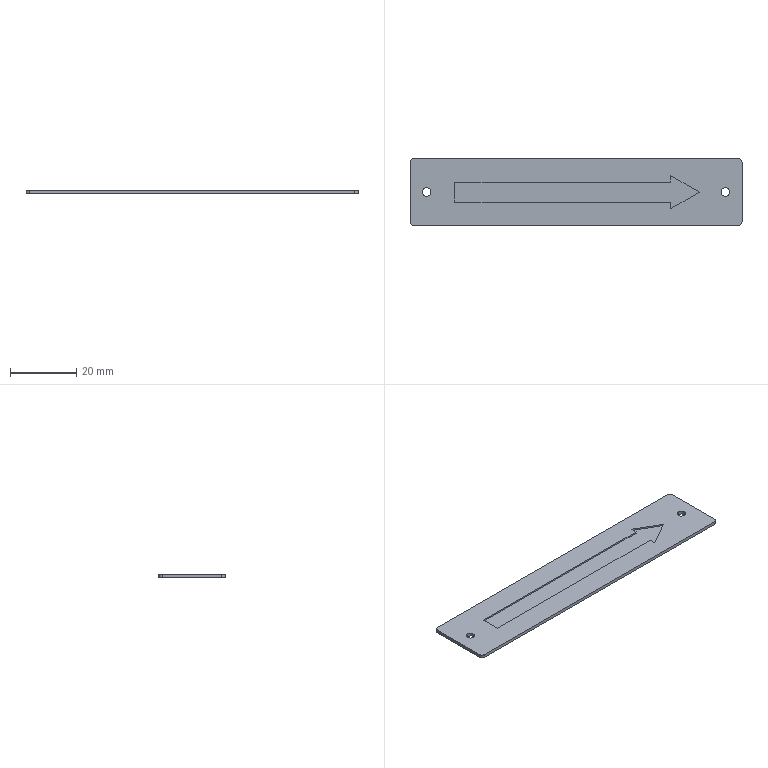Part | STEP file | [Flow direction nameplate]-Part-2 | 1 solid | 22 faces | box 100 x 20 x 1 mm | volume 1794 mm3 | plane 14 | cylinder 8 | commonest cylinder face diameters 2 x4 2.5 x4
STEP:
#1=CARTESIAN_POINT('',(-320.023,-38.283,51.8));
#2=VERTEX_POINT('',#1);
#3=CARTESIAN_POINT('',(-320.023,-35.783,51.8));
#4=VERTEX_POINT('',#3);
#5=CARTESIAN_POINT('',(-320.023,-37.033,51.8));
#6=DIRECTION('',(0.,0.,-1.));
#7=DIRECTION('',(0.,1.,0.));
#8=AXIS2_PLACEMENT_3D('',#5,#6,#7);
#9=CIRCLE('',#8,1.25);
#10=EDGE_CURVE('',#2,#4,#9,.T.);
#11=ORIENTED_EDGE('',*,*,#10,.F.);
#12=CARTESIAN_POINT('',(-320.023,-38.283,50.8));
#13=VERTEX_POINT('',#12);
#14=CARTESIAN_POINT('',(-320.023,-38.283,51.8));
#15=DIRECTION('',(0.,0.,-1.));
#16=VECTOR('',#15,1000.);
#17=LINE('',#14,#16);
#18=EDGE_CURVE('',#2,#13,#17,.T.);
#19=ORIENTED_EDGE('',*,*,#18,.T.);
#20=CARTESIAN_POINT('',(-320.023,-35.783,50.8));
#21=VERTEX_POINT('',#20);
#22=CARTESIAN_POINT('',(-320.023,-37.033,50.8));
#23=DIRECTION('',(0.,0.,1.));
#24=DIRECTION('',(0.,-1.,0.));
#25=AXIS2_PLACEMENT_3D('',#22,#23,#24);
#26=CIRCLE('',#25,1.25);
#27=EDGE_CURVE('',#21,#13,#26,.T.);
#28=ORIENTED_EDGE('',*,*,#27,.F.);
#29=CARTESIAN_POINT('',(-320.023,-35.783,51.8));
#30=DIRECTION('',(0.,0.,-1.));
#31=VECTOR('',#30,1000.);
#32=LINE('',#29,#31);
#33=EDGE_CURVE('',#4,#21,#32,.T.);
#34=ORIENTED_EDGE('',*,*,#33,.F.);
#35=EDGE_LOOP('',(#11,#19,#28,#34));
#36=FACE_OUTER_BOUND('',#35,.T.);
#37=CARTESIAN_POINT('',(-320.023,-37.033,51.8));
#38=DIRECTION('',(0.,0.,-1.));
#39=DIRECTION('',(0.,1.,0.));
#40=AXIS2_PLACEMENT_3D('',#37,#38,#39);
#41=CYLINDRICAL_SURFACE('',#40,1.25);
#42=ADVANCED_FACE('',(#36),#41,.F.);
#43=CARTESIAN_POINT('',(-230.023,-38.283,51.8));
#44=VERTEX_POINT('',#43);
#45=CARTESIAN_POINT('',(-230.023,-35.783,51.8));
#46=VERTEX_POINT('',#45);
#47=CARTESIAN_POINT('',(-230.023,-37.033,51.8));
#48=DIRECTION('',(0.,0.,-1.));
#49=DIRECTION('',(0.,1.,0.));
#50=AXIS2_PLACEMENT_3D('',#47,#48,#49);
#51=CIRCLE('',#50,1.25);
#52=EDGE_CURVE('',#44,#46,#51,.T.);
#53=ORIENTED_EDGE('',*,*,#52,.F.);
#54=CARTESIAN_POINT('',(-230.023,-38.283,50.8));
#55=VERTEX_POINT('',#54);
#56=CARTESIAN_POINT('',(-230.023,-38.283,51.8));
#57=DIRECTION('',(0.,0.,-1.));
#58=VECTOR('',#57,1000.);
#59=LINE('',#56,#58);
#60=EDGE_CURVE('',#44,#55,#59,.T.);
#61=ORIENTED_EDGE('',*,*,#60,.T.);
#62=CARTESIAN_POINT('',(-230.023,-35.783,50.8));
#63=VERTEX_POINT('',#62);
#64=CARTESIAN_POINT('',(-230.023,-37.033,50.8));
#65=DIRECTION('',(0.,0.,1.));
#66=DIRECTION('',(0.,-1.,0.));
#67=AXIS2_PLACEMENT_3D('',#64,#65,#66);
#68=CIRCLE('',#67,1.25);
#69=EDGE_CURVE('',#63,#55,#68,.T.);
#70=ORIENTED_EDGE('',*,*,#69,.F.);
#71=CARTESIAN_POINT('',(-230.023,-35.783,51.8));
#72=DIRECTION('',(0.,0.,-1.));
#73=VECTOR('',#72,1000.);
#74=LINE('',#71,#73);
#75=EDGE_CURVE('',#46,#63,#74,.T.);
#76=ORIENTED_EDGE('',*,*,#75,.F.);
#77=EDGE_LOOP('',(#53,#61,#70,#76));
#78=FACE_OUTER_BOUND('',#77,.T.);
#79=CARTESIAN_POINT('',(-230.023,-37.033,51.8));
#80=DIRECTION('',(0.,0.,-1.));
#81=DIRECTION('',(0.,1.,0.));
#82=AXIS2_PLACEMENT_3D('',#79,#80,#81);
#83=CYLINDRICAL_SURFACE('',#82,1.25);
#84=ADVANCED_FACE('',(#78),#83,.F.);
#85=CARTESIAN_POINT('',(-324.023,-27.033,50.8));
#86=VERTEX_POINT('',#85);
#87=CARTESIAN_POINT('',(-226.023,-27.033,50.8));
#88=VERTEX_POINT('',#87);
#89=CARTESIAN_POINT('',(-275.023,-27.033,50.8));
#90=DIRECTION('',(1.,0.,0.));
#91=VECTOR('',#90,1000.);
#92=LINE('',#89,#91);
#93=EDGE_CURVE('',#86,#88,#92,.T.);
#94=ORIENTED_EDGE('',*,*,#93,.F.);
#95=CARTESIAN_POINT('',(-324.023,-27.033,51.8));
#96=VERTEX_POINT('',#95);
#97=CARTESIAN_POINT('',(-324.023,-27.033,51.3));
#98=DIRECTION('',(0.,0.,1.));
#99=VECTOR('',#98,1000.);
#100=LINE('',#97,#99);
#101=EDGE_CURVE('',#86,#96,#100,.T.);
#102=ORIENTED_EDGE('',*,*,#101,.T.);
#103=CARTESIAN_POINT('',(-226.023,-27.033,51.8));
#104=VERTEX_POINT('',#103);
#105=CARTESIAN_POINT('',(-275.023,-27.033,51.8));
#106=DIRECTION('',(-1.,0.,0.));
#107=VECTOR('',#106,1000.);
#108=LINE('',#105,#107);
#109=EDGE_CURVE('',#104,#96,#108,.T.);
#110=ORIENTED_EDGE('',*,*,#109,.F.);
#111=CARTESIAN_POINT('',(-226.023,-27.033,51.3));
#112=DIRECTION('',(0.,0.,-1.));
#113=VECTOR('',#112,1000.);
#114=LINE('',#111,#113);
#115=EDGE_CURVE('',#104,#88,#114,.T.);
#116=ORIENTED_EDGE('',*,*,#115,.T.);
#117=EDGE_LOOP('',(#94,#102,#110,#116));
#118=FACE_OUTER_BOUND('',#117,.T.);
#119=CARTESIAN_POINT('',(-275.023,-27.033,51.3));
#120=DIRECTION('',(0.,1.,0.));
#121=DIRECTION('',(1.,0.,0.));
#122=AXIS2_PLACEMENT_3D('',#119,#120,#121);
#123=PLANE('',#122);
#124=ADVANCED_FACE('',(#118),#123,.T.);
#125=CARTESIAN_POINT('',(-311.498,-40.081,51.8));
#126=VERTEX_POINT('',#125);
#127=CARTESIAN_POINT('',(-311.498,-34.081,51.8));
#128=VERTEX_POINT('',#127);
#129=CARTESIAN_POINT('',(-311.498,-47.033,51.8));
#130=DIRECTION('',(0.,1.,0.));
#131=VECTOR('',#130,1000.);
#132=LINE('',#129,#131);
#133=EDGE_CURVE('',#126,#128,#132,.T.);
#134=ORIENTED_EDGE('',*,*,#133,.T.);
#135=CARTESIAN_POINT('',(-246.498,-34.081,51.8));
#136=VERTEX_POINT('',#135);
#137=CARTESIAN_POINT('',(-275.023,-34.081,51.8));
#138=DIRECTION('',(1.,0.,0.));
#139=VECTOR('',#138,1000.);
#140=LINE('',#137,#139);
#141=EDGE_CURVE('',#128,#136,#140,.T.);
#142=ORIENTED_EDGE('',*,*,#141,.T.);
#143=CARTESIAN_POINT('',(-246.498,-32.081,51.8));
#144=VERTEX_POINT('',#143);
#145=CARTESIAN_POINT('',(-246.498,-47.033,51.8));
#146=DIRECTION('',(0.,1.,0.));
#147=VECTOR('',#146,1000.);
#148=LINE('',#145,#147);
#149=EDGE_CURVE('',#136,#144,#148,.T.);
#150=ORIENTED_EDGE('',*,*,#149,.T.);
#151=CARTESIAN_POINT('',(-237.838,-37.081,51.8));
#152=VERTEX_POINT('',#151);
#153=CARTESIAN_POINT('',(-261.417,-23.467,51.8));
#154=DIRECTION('',(0.866,-0.5,0.));
#155=VECTOR('',#154,1000.);
#156=LINE('',#153,#155);
#157=EDGE_CURVE('',#144,#152,#156,.T.);
#158=ORIENTED_EDGE('',*,*,#157,.T.);
#159=CARTESIAN_POINT('',(-246.498,-42.081,51.8));
#160=VERTEX_POINT('',#159);
#161=CARTESIAN_POINT('',(-270.036,-55.67,51.8));
#162=DIRECTION('',(-0.866,-0.5,0.));
#163=VECTOR('',#162,1000.);
#164=LINE('',#161,#163);
#165=EDGE_CURVE('',#152,#160,#164,.T.);
#166=ORIENTED_EDGE('',*,*,#165,.T.);
#167=CARTESIAN_POINT('',(-246.498,-40.081,51.8));
#168=VERTEX_POINT('',#167);
#169=CARTESIAN_POINT('',(-246.498,-47.033,51.8));
#170=DIRECTION('',(0.,1.,0.));
#171=VECTOR('',#170,1000.);
#172=LINE('',#169,#171);
#173=EDGE_CURVE('',#160,#168,#172,.T.);
#174=ORIENTED_EDGE('',*,*,#173,.T.);
#175=CARTESIAN_POINT('',(-275.023,-40.081,51.8));
#176=DIRECTION('',(-1.,0.,0.));
#177=VECTOR('',#176,1000.);
#178=LINE('',#175,#177);
#179=EDGE_CURVE('',#168,#126,#178,.T.);
#180=ORIENTED_EDGE('',*,*,#179,.T.);
#181=EDGE_LOOP('',(#134,#142,#150,#158,#166,#174,#180));
#182=FACE_BOUND('',#181,.T.);
#183=CARTESIAN_POINT('',(-320.023,-37.033,51.8));
#184=DIRECTION('',(0.,0.,-1.));
#185=DIRECTION('',(0.,1.,0.));
#186=AXIS2_PLACEMENT_3D('',#183,#184,#185);
#187=CIRCLE('',#186,1.25);
#188=EDGE_CURVE('',#4,#2,#187,.T.);
#189=ORIENTED_EDGE('',*,*,#188,.T.);
#190=ORIENTED_EDGE('',*,*,#10,.T.);
#191=EDGE_LOOP('',(#189,#190));
#192=FACE_BOUND('',#191,.T.);
#193=CARTESIAN_POINT('',(-230.023,-37.033,51.8));
#194=DIRECTION('',(0.,0.,-1.));
#195=DIRECTION('',(0.,1.,0.));
#196=AXIS2_PLACEMENT_3D('',#193,#194,#195);
#197=CIRCLE('',#196,1.25);
#198=EDGE_CURVE('',#46,#44,#197,.T.);
#199=ORIENTED_EDGE('',*,*,#198,.T.);
#200=ORIENTED_EDGE('',*,*,#52,.T.);
#201=EDGE_LOOP('',(#199,#200));
#202=FACE_BOUND('',#201,.T.);
#203=CARTESIAN_POINT('',(-325.023,-46.033,51.8));
#204=VERTEX_POINT('',#203);
#205=CARTESIAN_POINT('',(-325.023,-28.033,51.8));
#206=VERTEX_POINT('',#205);
#207=CARTESIAN_POINT('',(-325.023,-47.033,51.8));
#208=DIRECTION('',(0.,1.,0.));
#209=VECTOR('',#208,1000.);
#210=LINE('',#207,#209);
#211=EDGE_CURVE('',#204,#206,#210,.T.);
#212=ORIENTED_EDGE('',*,*,#211,.F.);
#213=CARTESIAN_POINT('',(-324.023,-47.033,51.8));
#214=VERTEX_POINT('',#213);
#215=CARTESIAN_POINT('',(-324.023,-46.033,51.8));
#216=DIRECTION('',(0.,0.,1.));
#217=DIRECTION('',(0.,-1.,0.));
#218=AXIS2_PLACEMENT_3D('',#215,#216,#217);
#219=CIRCLE('',#218,1.);
#220=EDGE_CURVE('',#204,#214,#219,.T.);
#221=ORIENTED_EDGE('',*,*,#220,.T.);
#222=CARTESIAN_POINT('',(-226.023,-47.033,51.8));
#223=VERTEX_POINT('',#222);
#224=CARTESIAN_POINT('',(-275.023,-47.033,51.8));
#225=DIRECTION('',(1.,0.,0.));
#226=VECTOR('',#225,1000.);
#227=LINE('',#224,#226);
#228=EDGE_CURVE('',#214,#223,#227,.T.);
#229=ORIENTED_EDGE('',*,*,#228,.T.);
#230=CARTESIAN_POINT('',(-225.023,-46.033,51.8));
#231=VERTEX_POINT('',#230);
#232=CARTESIAN_POINT('',(-226.023,-46.033,51.8));
#233=DIRECTION('',(0.,0.,1.));
#234=DIRECTION('',(0.,-1.,0.));
#235=AXIS2_PLACEMENT_3D('',#232,#233,#234);
#236=CIRCLE('',#235,1.);
#237=EDGE_CURVE('',#223,#231,#236,.T.);
#238=ORIENTED_EDGE('',*,*,#237,.T.);
#239=CARTESIAN_POINT('',(-225.023,-28.033,51.8));
#240=VERTEX_POINT('',#239);
#241=CARTESIAN_POINT('',(-225.023,-47.033,51.8));
#242=DIRECTION('',(0.,1.,0.));
#243=VECTOR('',#242,1000.);
#244=LINE('',#241,#243);
#245=EDGE_CURVE('',#231,#240,#244,.T.);
#246=ORIENTED_EDGE('',*,*,#245,.T.);
#247=CARTESIAN_POINT('',(-226.023,-28.033,51.8));
#248=DIRECTION('',(0.,0.,1.));
#249=DIRECTION('',(0.,-1.,0.));
#250=AXIS2_PLACEMENT_3D('',#247,#248,#249);
#251=CIRCLE('',#250,1.);
#252=EDGE_CURVE('',#240,#104,#251,.T.);
#253=ORIENTED_EDGE('',*,*,#252,.T.);
#254=ORIENTED_EDGE('',*,*,#109,.T.);
#255=CARTESIAN_POINT('',(-324.023,-28.033,51.8));
#256=DIRECTION('',(0.,0.,1.));
#257=DIRECTION('',(0.,-1.,0.));
#258=AXIS2_PLACEMENT_3D('',#255,#256,#257);
#259=CIRCLE('',#258,1.);
#260=EDGE_CURVE('',#96,#206,#259,.T.);
#261=ORIENTED_EDGE('',*,*,#260,.T.);
#262=EDGE_LOOP('',(#212,#221,#229,#238,#246,#253,#254,#261));
#263=FACE_OUTER_BOUND('',#262,.T.);
#264=CARTESIAN_POINT('',(-275.023,-47.033,51.8));
#265=DIRECTION('',(0.,0.,1.));
#266=DIRECTION('',(0.,-1.,0.));
#267=AXIS2_PLACEMENT_3D('',#264,#265,#266);
#268=PLANE('',#267);
#269=ADVANCED_FACE('',(#182,#192,#202,#263),#268,.T.);
#270=CARTESIAN_POINT('',(-325.023,-46.033,50.8));
#271=VERTEX_POINT('',#270);
#272=CARTESIAN_POINT('',(-325.023,-28.033,50.8));
#273=VERTEX_POINT('',#272);
#274=CARTESIAN_POINT('',(-325.023,-47.033,50.8));
#275=DIRECTION('',(0.,1.,0.));
#276=VECTOR('',#275,1000.);
#277=LINE('',#274,#276);
#278=EDGE_CURVE('',#271,#273,#277,.T.);
#279=ORIENTED_EDGE('',*,*,#278,.F.);
#280=CARTESIAN_POINT('',(-325.023,-46.033,51.3));
#281=DIRECTION('',(0.,0.,1.));
#282=VECTOR('',#281,1000.);
#283=LINE('',#280,#282);
#284=EDGE_CURVE('',#271,#204,#283,.T.);
#285=ORIENTED_EDGE('',*,*,#284,.T.);
#286=ORIENTED_EDGE('',*,*,#211,.T.);
#287=CARTESIAN_POINT('',(-325.023,-28.033,51.3));
#288=DIRECTION('',(0.,0.,-1.));
#289=VECTOR('',#288,1000.);
#290=LINE('',#287,#289);
#291=EDGE_CURVE('',#206,#273,#290,.T.);
#292=ORIENTED_EDGE('',*,*,#291,.T.);
#293=EDGE_LOOP('',(#279,#285,#286,#292));
#294=FACE_OUTER_BOUND('',#293,.T.);
#295=CARTESIAN_POINT('',(-325.023,-47.033,51.3));
#296=DIRECTION('',(-1.,0.,0.));
#297=DIRECTION('',(0.,1.,0.));
#298=AXIS2_PLACEMENT_3D('',#295,#296,#297);
#299=PLANE('',#298);
#300=ADVANCED_FACE('',(#294),#299,.T.);
#301=ORIENTED_EDGE('',*,*,#27,.T.);
#302=CARTESIAN_POINT('',(-320.023,-37.033,50.8));
#303=DIRECTION('',(0.,0.,1.));
#304=DIRECTION('',(0.,-1.,0.));
#305=AXIS2_PLACEMENT_3D('',#302,#303,#304);
#306=CIRCLE('',#305,1.25);
#307=EDGE_CURVE('',#13,#21,#306,.T.);
#308=ORIENTED_EDGE('',*,*,#307,.T.);
#309=EDGE_LOOP('',(#301,#308));
#310=FACE_BOUND('',#309,.T.);
#311=ORIENTED_EDGE('',*,*,#69,.T.);
#312=CARTESIAN_POINT('',(-230.023,-37.033,50.8));
#313=DIRECTION('',(0.,0.,1.));
#314=DIRECTION('',(0.,-1.,0.));
#315=AXIS2_PLACEMENT_3D('',#312,#313,#314);
#316=CIRCLE('',#315,1.25);
#317=EDGE_CURVE('',#55,#63,#316,.T.);
#318=ORIENTED_EDGE('',*,*,#317,.T.);
#319=EDGE_LOOP('',(#311,#318));
#320=FACE_BOUND('',#319,.T.);
#321=CARTESIAN_POINT('',(-226.023,-47.033,50.8));
#322=VERTEX_POINT('',#321);
#323=CARTESIAN_POINT('',(-324.023,-47.033,50.8));
#324=VERTEX_POINT('',#323);
#325=CARTESIAN_POINT('',(-275.023,-47.033,50.8));
#326=DIRECTION('',(-1.,0.,0.));
#327=VECTOR('',#326,1000.);
#328=LINE('',#325,#327);
#329=EDGE_CURVE('',#322,#324,#328,.T.);
#330=ORIENTED_EDGE('',*,*,#329,.T.);
#331=CARTESIAN_POINT('',(-324.023,-46.033,50.8));
#332=DIRECTION('',(0.,0.,-1.));
#333=DIRECTION('',(0.,1.,0.));
#334=AXIS2_PLACEMENT_3D('',#331,#332,#333);
#335=CIRCLE('',#334,1.);
#336=EDGE_CURVE('',#324,#271,#335,.T.);
#337=ORIENTED_EDGE('',*,*,#336,.T.);
#338=ORIENTED_EDGE('',*,*,#278,.T.);
#339=CARTESIAN_POINT('',(-324.023,-28.033,50.8));
#340=DIRECTION('',(0.,0.,-1.));
#341=DIRECTION('',(0.,1.,0.));
#342=AXIS2_PLACEMENT_3D('',#339,#340,#341);
#343=CIRCLE('',#342,1.);
#344=EDGE_CURVE('',#273,#86,#343,.T.);
#345=ORIENTED_EDGE('',*,*,#344,.T.);
#346=ORIENTED_EDGE('',*,*,#93,.T.);
#347=CARTESIAN_POINT('',(-225.023,-28.033,50.8));
#348=VERTEX_POINT('',#347);
#349=CARTESIAN_POINT('',(-226.023,-28.033,50.8));
#350=DIRECTION('',(0.,0.,-1.));
#351=DIRECTION('',(0.,1.,0.));
#352=AXIS2_PLACEMENT_3D('',#349,#350,#351);
#353=CIRCLE('',#352,1.);
#354=EDGE_CURVE('',#88,#348,#353,.T.);
#355=ORIENTED_EDGE('',*,*,#354,.T.);
#356=CARTESIAN_POINT('',(-225.023,-46.033,50.8));
#357=VERTEX_POINT('',#356);
#358=CARTESIAN_POINT('',(-225.023,-47.033,50.8));
#359=DIRECTION('',(0.,1.,0.));
#360=VECTOR('',#359,1000.);
#361=LINE('',#358,#360);
#362=EDGE_CURVE('',#357,#348,#361,.T.);
#363=ORIENTED_EDGE('',*,*,#362,.F.);
#364=CARTESIAN_POINT('',(-226.023,-46.033,50.8));
#365=DIRECTION('',(0.,0.,-1.));
#366=DIRECTION('',(0.,1.,0.));
#367=AXIS2_PLACEMENT_3D('',#364,#365,#366);
#368=CIRCLE('',#367,1.);
#369=EDGE_CURVE('',#357,#322,#368,.T.);
#370=ORIENTED_EDGE('',*,*,#369,.T.);
#371=EDGE_LOOP('',(#330,#337,#338,#345,#346,#355,#363,#370));
#372=FACE_OUTER_BOUND('',#371,.T.);
#373=CARTESIAN_POINT('',(-275.023,-47.033,50.8));
#374=DIRECTION('',(0.,0.,-1.));
#375=DIRECTION('',(0.,1.,0.));
#376=AXIS2_PLACEMENT_3D('',#373,#374,#375);
#377=PLANE('',#376);
#378=ADVANCED_FACE('',(#310,#320,#372),#377,.T.);
#379=ORIENTED_EDGE('',*,*,#228,.F.);
#380=CARTESIAN_POINT('',(-324.023,-47.033,51.3));
#381=DIRECTION('',(0.,0.,-1.));
#382=VECTOR('',#381,1000.);
#383=LINE('',#380,#382);
#384=EDGE_CURVE('',#214,#324,#383,.T.);
#385=ORIENTED_EDGE('',*,*,#384,.T.);
#386=ORIENTED_EDGE('',*,*,#329,.F.);
#387=CARTESIAN_POINT('',(-226.023,-47.033,51.3));
#388=DIRECTION('',(0.,0.,1.));
#389=VECTOR('',#388,1000.);
#390=LINE('',#387,#389);
#391=EDGE_CURVE('',#322,#223,#390,.T.);
#392=ORIENTED_EDGE('',*,*,#391,.T.);
#393=EDGE_LOOP('',(#379,#385,#386,#392));
#394=FACE_OUTER_BOUND('',#393,.T.);
#395=CARTESIAN_POINT('',(-275.023,-47.033,51.3));
#396=DIRECTION('',(0.,-1.,0.));
#397=DIRECTION('',(-1.,0.,0.));
#398=AXIS2_PLACEMENT_3D('',#395,#396,#397);
#399=PLANE('',#398);
#400=ADVANCED_FACE('',(#394),#399,.T.);
#401=ORIENTED_EDGE('',*,*,#362,.T.);
#402=CARTESIAN_POINT('',(-225.023,-28.033,51.3));
#403=DIRECTION('',(0.,0.,1.));
#404=VECTOR('',#403,1000.);
#405=LINE('',#402,#404);
#406=EDGE_CURVE('',#348,#240,#405,.T.);
#407=ORIENTED_EDGE('',*,*,#406,.T.);
#408=ORIENTED_EDGE('',*,*,#245,.F.);
#409=CARTESIAN_POINT('',(-225.023,-46.033,51.3));
#410=DIRECTION('',(0.,0.,-1.));
#411=VECTOR('',#410,1000.);
#412=LINE('',#409,#411);
#413=EDGE_CURVE('',#231,#357,#412,.T.);
#414=ORIENTED_EDGE('',*,*,#413,.T.);
#415=EDGE_LOOP('',(#401,#407,#408,#414));
#416=FACE_OUTER_BOUND('',#415,.T.);
#417=CARTESIAN_POINT('',(-225.023,-47.033,51.3));
#418=DIRECTION('',(1.,0.,0.));
#419=DIRECTION('',(0.,-1.,0.));
#420=AXIS2_PLACEMENT_3D('',#417,#418,#419);
#421=PLANE('',#420);
#422=ADVANCED_FACE('',(#416),#421,.T.);
#423=ORIENTED_EDGE('',*,*,#60,.F.);
#424=ORIENTED_EDGE('',*,*,#198,.F.);
#425=ORIENTED_EDGE('',*,*,#75,.T.);
#426=ORIENTED_EDGE('',*,*,#317,.F.);
#427=EDGE_LOOP('',(#423,#424,#425,#426));
#428=FACE_OUTER_BOUND('',#427,.T.);
#429=CARTESIAN_POINT('',(-230.023,-37.033,51.8));
#430=DIRECTION('',(0.,0.,-1.));
#431=DIRECTION('',(0.,1.,0.));
#432=AXIS2_PLACEMENT_3D('',#429,#430,#431);
#433=CYLINDRICAL_SURFACE('',#432,1.25);
#434=ADVANCED_FACE('',(#428),#433,.F.);
#435=ORIENTED_EDGE('',*,*,#18,.F.);
#436=ORIENTED_EDGE('',*,*,#188,.F.);
#437=ORIENTED_EDGE('',*,*,#33,.T.);
#438=ORIENTED_EDGE('',*,*,#307,.F.);
#439=EDGE_LOOP('',(#435,#436,#437,#438));
#440=FACE_OUTER_BOUND('',#439,.T.);
#441=CARTESIAN_POINT('',(-320.023,-37.033,51.8));
#442=DIRECTION('',(0.,0.,-1.));
#443=DIRECTION('',(0.,1.,0.));
#444=AXIS2_PLACEMENT_3D('',#441,#442,#443);
#445=CYLINDRICAL_SURFACE('',#444,1.25);
#446=ADVANCED_FACE('',(#440),#445,.F.);
#447=ORIENTED_EDGE('',*,*,#237,.F.);
#448=ORIENTED_EDGE('',*,*,#391,.F.);
#449=ORIENTED_EDGE('',*,*,#369,.F.);
#450=ORIENTED_EDGE('',*,*,#413,.F.);
#451=EDGE_LOOP('',(#447,#448,#449,#450));
#452=FACE_OUTER_BOUND('',#451,.T.);
#453=CARTESIAN_POINT('',(-226.023,-46.033,51.3));
#454=DIRECTION('',(0.,0.,-1.));
#455=DIRECTION('',(0.,1.,0.));
#456=AXIS2_PLACEMENT_3D('',#453,#454,#455);
#457=CYLINDRICAL_SURFACE('',#456,1.);
#458=ADVANCED_FACE('',(#452),#457,.T.);
#459=ORIENTED_EDGE('',*,*,#354,.F.);
#460=ORIENTED_EDGE('',*,*,#115,.F.);
#461=ORIENTED_EDGE('',*,*,#252,.F.);
#462=ORIENTED_EDGE('',*,*,#406,.F.);
#463=EDGE_LOOP('',(#459,#460,#461,#462));
#464=FACE_OUTER_BOUND('',#463,.T.);
#465=CARTESIAN_POINT('',(-226.023,-28.033,51.3));
#466=DIRECTION('',(0.,0.,1.));
#467=DIRECTION('',(0.,-1.,0.));
#468=AXIS2_PLACEMENT_3D('',#465,#466,#467);
#469=CYLINDRICAL_SURFACE('',#468,1.);
#470=ADVANCED_FACE('',(#464),#469,.T.);
#471=ORIENTED_EDGE('',*,*,#260,.F.);
#472=ORIENTED_EDGE('',*,*,#101,.F.);
#473=ORIENTED_EDGE('',*,*,#344,.F.);
#474=ORIENTED_EDGE('',*,*,#291,.F.);
#475=EDGE_LOOP('',(#471,#472,#473,#474));
#476=FACE_OUTER_BOUND('',#475,.T.);
#477=CARTESIAN_POINT('',(-324.023,-28.033,51.3));
#478=DIRECTION('',(0.,0.,-1.));
#479=DIRECTION('',(0.,1.,0.));
#480=AXIS2_PLACEMENT_3D('',#477,#478,#479);
#481=CYLINDRICAL_SURFACE('',#480,1.);
#482=ADVANCED_FACE('',(#476),#481,.T.);
#483=ORIENTED_EDGE('',*,*,#336,.F.);
#484=ORIENTED_EDGE('',*,*,#384,.F.);
#485=ORIENTED_EDGE('',*,*,#220,.F.);
#486=ORIENTED_EDGE('',*,*,#284,.F.);
#487=EDGE_LOOP('',(#483,#484,#485,#486));
#488=FACE_OUTER_BOUND('',#487,.T.);
#489=CARTESIAN_POINT('',(-324.023,-46.033,51.3));
#490=DIRECTION('',(0.,0.,1.));
#491=DIRECTION('',(0.,-1.,0.));
#492=AXIS2_PLACEMENT_3D('',#489,#490,#491);
#493=CYLINDRICAL_SURFACE('',#492,1.);
#494=ADVANCED_FACE('',(#488),#493,.T.);
#495=ORIENTED_EDGE('',*,*,#133,.F.);
#496=CARTESIAN_POINT('',(-311.498,-40.081,51.35));
#497=VERTEX_POINT('',#496);
#498=CARTESIAN_POINT('',(-311.498,-40.081,51.85));
#499=DIRECTION('',(0.,0.,-1.));
#500=VECTOR('',#499,1000.);
#501=LINE('',#498,#500);
#502=EDGE_CURVE('',#126,#497,#501,.T.);
#503=ORIENTED_EDGE('',*,*,#502,.T.);
#504=CARTESIAN_POINT('',(-311.498,-34.081,51.35));
#505=VERTEX_POINT('',#504);
#506=CARTESIAN_POINT('',(-311.498,-34.081,51.35));
#507=DIRECTION('',(0.,-1.,0.));
#508=VECTOR('',#507,1000.);
#509=LINE('',#506,#508);
#510=EDGE_CURVE('',#505,#497,#509,.T.);
#511=ORIENTED_EDGE('',*,*,#510,.F.);
#512=CARTESIAN_POINT('',(-311.498,-34.081,51.85));
#513=DIRECTION('',(0.,0.,-1.));
#514=VECTOR('',#513,1000.);
#515=LINE('',#512,#514);
#516=EDGE_CURVE('',#128,#505,#515,.T.);
#517=ORIENTED_EDGE('',*,*,#516,.F.);
#518=EDGE_LOOP('',(#495,#503,#511,#517));
#519=FACE_OUTER_BOUND('',#518,.T.);
#520=CARTESIAN_POINT('',(-311.498,-34.081,51.85));
#521=DIRECTION('',(-1.,0.,0.));
#522=DIRECTION('',(0.,0.,-1.));
#523=AXIS2_PLACEMENT_3D('',#520,#521,#522);
#524=PLANE('',#523);
#525=ADVANCED_FACE('',(#519),#524,.F.);
#526=ORIENTED_EDGE('',*,*,#179,.F.);
#527=CARTESIAN_POINT('',(-246.498,-40.081,51.35));
#528=VERTEX_POINT('',#527);
#529=CARTESIAN_POINT('',(-246.498,-40.081,51.85));
#530=DIRECTION('',(0.,0.,-1.));
#531=VECTOR('',#530,1000.);
#532=LINE('',#529,#531);
#533=EDGE_CURVE('',#168,#528,#532,.T.);
#534=ORIENTED_EDGE('',*,*,#533,.T.);
#535=CARTESIAN_POINT('',(-311.498,-40.081,51.35));
#536=DIRECTION('',(1.,0.,0.));
#537=VECTOR('',#536,1000.);
#538=LINE('',#535,#537);
#539=EDGE_CURVE('',#497,#528,#538,.T.);
#540=ORIENTED_EDGE('',*,*,#539,.F.);
#541=ORIENTED_EDGE('',*,*,#502,.F.);
#542=EDGE_LOOP('',(#526,#534,#540,#541));
#543=FACE_OUTER_BOUND('',#542,.T.);
#544=CARTESIAN_POINT('',(-311.498,-40.081,51.85));
#545=DIRECTION('',(0.,-1.,0.));
#546=DIRECTION('',(0.,0.,-1.));
#547=AXIS2_PLACEMENT_3D('',#544,#545,#546);
#548=PLANE('',#547);
#549=ADVANCED_FACE('',(#543),#548,.F.);
#550=ORIENTED_EDGE('',*,*,#173,.F.);
#551=CARTESIAN_POINT('',(-246.498,-42.081,51.35));
#552=VERTEX_POINT('',#551);
#553=CARTESIAN_POINT('',(-246.498,-42.081,51.85));
#554=DIRECTION('',(0.,0.,-1.));
#555=VECTOR('',#554,1000.);
#556=LINE('',#553,#555);
#557=EDGE_CURVE('',#160,#552,#556,.T.);
#558=ORIENTED_EDGE('',*,*,#557,.T.);
#559=CARTESIAN_POINT('',(-246.498,-40.081,51.35));
#560=DIRECTION('',(0.,-1.,0.));
#561=VECTOR('',#560,1000.);
#562=LINE('',#559,#561);
#563=EDGE_CURVE('',#528,#552,#562,.T.);
#564=ORIENTED_EDGE('',*,*,#563,.F.);
#565=ORIENTED_EDGE('',*,*,#533,.F.);
#566=EDGE_LOOP('',(#550,#558,#564,#565));
#567=FACE_OUTER_BOUND('',#566,.T.);
#568=CARTESIAN_POINT('',(-246.498,-40.081,51.85));
#569=DIRECTION('',(-1.,0.,0.));
#570=DIRECTION('',(0.,0.,-1.));
#571=AXIS2_PLACEMENT_3D('',#568,#569,#570);
#572=PLANE('',#571);
#573=ADVANCED_FACE('',(#567),#572,.F.);
#574=ORIENTED_EDGE('',*,*,#165,.F.);
#575=CARTESIAN_POINT('',(-237.838,-37.081,51.35));
#576=VERTEX_POINT('',#575);
#577=CARTESIAN_POINT('',(-237.838,-37.081,51.85));
#578=DIRECTION('',(0.,0.,-1.));
#579=VECTOR('',#578,1000.);
#580=LINE('',#577,#579);
#581=EDGE_CURVE('',#152,#576,#580,.T.);
#582=ORIENTED_EDGE('',*,*,#581,.T.);
#583=CARTESIAN_POINT('',(-246.498,-42.081,51.35));
#584=DIRECTION('',(0.866,0.5,0.));
#585=VECTOR('',#584,1000.);
#586=LINE('',#583,#585);
#587=EDGE_CURVE('',#552,#576,#586,.T.);
#588=ORIENTED_EDGE('',*,*,#587,.F.);
#589=ORIENTED_EDGE('',*,*,#557,.F.);
#590=EDGE_LOOP('',(#574,#582,#588,#589));
#591=FACE_OUTER_BOUND('',#590,.T.);
#592=CARTESIAN_POINT('',(-246.498,-42.081,51.85));
#593=DIRECTION('',(0.5,-0.866,0.));
#594=DIRECTION('',(0.866,0.5,0.));
#595=AXIS2_PLACEMENT_3D('',#592,#593,#594);
#596=PLANE('',#595);
#597=ADVANCED_FACE('',(#591),#596,.F.);
#598=ORIENTED_EDGE('',*,*,#157,.F.);
#599=CARTESIAN_POINT('',(-246.498,-32.081,51.35));
#600=VERTEX_POINT('',#599);
#601=CARTESIAN_POINT('',(-246.498,-32.081,51.85));
#602=DIRECTION('',(0.,0.,-1.));
#603=VECTOR('',#602,1000.);
#604=LINE('',#601,#603);
#605=EDGE_CURVE('',#144,#600,#604,.T.);
#606=ORIENTED_EDGE('',*,*,#605,.T.);
#607=CARTESIAN_POINT('',(-237.838,-37.081,51.35));
#608=DIRECTION('',(-0.866,0.5,0.));
#609=VECTOR('',#608,1000.);
#610=LINE('',#607,#609);
#611=EDGE_CURVE('',#576,#600,#610,.T.);
#612=ORIENTED_EDGE('',*,*,#611,.F.);
#613=ORIENTED_EDGE('',*,*,#581,.F.);
#614=EDGE_LOOP('',(#598,#606,#612,#613));
#615=FACE_OUTER_BOUND('',#614,.T.);
#616=CARTESIAN_POINT('',(-237.838,-37.081,51.85));
#617=DIRECTION('',(0.5,0.866,0.));
#618=DIRECTION('',(-0.866,0.5,0.));
#619=AXIS2_PLACEMENT_3D('',#616,#617,#618);
#620=PLANE('',#619);
#621=ADVANCED_FACE('',(#615),#620,.F.);
#622=ORIENTED_EDGE('',*,*,#149,.F.);
#623=CARTESIAN_POINT('',(-246.498,-34.081,51.35));
#624=VERTEX_POINT('',#623);
#625=CARTESIAN_POINT('',(-246.498,-34.081,51.85));
#626=DIRECTION('',(0.,0.,-1.));
#627=VECTOR('',#626,1000.);
#628=LINE('',#625,#627);
#629=EDGE_CURVE('',#136,#624,#628,.T.);
#630=ORIENTED_EDGE('',*,*,#629,.T.);
#631=CARTESIAN_POINT('',(-246.498,-32.081,51.35));
#632=DIRECTION('',(0.,-1.,0.));
#633=VECTOR('',#632,1000.);
#634=LINE('',#631,#633);
#635=EDGE_CURVE('',#600,#624,#634,.T.);
#636=ORIENTED_EDGE('',*,*,#635,.F.);
#637=ORIENTED_EDGE('',*,*,#605,.F.);
#638=EDGE_LOOP('',(#622,#630,#636,#637));
#639=FACE_OUTER_BOUND('',#638,.T.);
#640=CARTESIAN_POINT('',(-246.498,-32.081,51.85));
#641=DIRECTION('',(-1.,0.,0.));
#642=DIRECTION('',(0.,0.,-1.));
#643=AXIS2_PLACEMENT_3D('',#640,#641,#642);
#644=PLANE('',#643);
#645=ADVANCED_FACE('',(#639),#644,.F.);
#646=ORIENTED_EDGE('',*,*,#141,.F.);
#647=ORIENTED_EDGE('',*,*,#516,.T.);
#648=CARTESIAN_POINT('',(-246.498,-34.081,51.35));
#649=DIRECTION('',(-1.,0.,0.));
#650=VECTOR('',#649,1000.);
#651=LINE('',#648,#650);
#652=EDGE_CURVE('',#624,#505,#651,.T.);
#653=ORIENTED_EDGE('',*,*,#652,.F.);
#654=ORIENTED_EDGE('',*,*,#629,.F.);
#655=EDGE_LOOP('',(#646,#647,#653,#654));
#656=FACE_OUTER_BOUND('',#655,.T.);
#657=CARTESIAN_POINT('',(-246.498,-34.081,51.85));
#658=DIRECTION('',(0.,1.,0.));
#659=DIRECTION('',(0.,0.,1.));
#660=AXIS2_PLACEMENT_3D('',#657,#658,#659);
#661=PLANE('',#660);
#662=ADVANCED_FACE('',(#656),#661,.F.);
#663=ORIENTED_EDGE('',*,*,#510,.T.);
#664=ORIENTED_EDGE('',*,*,#539,.T.);
#665=ORIENTED_EDGE('',*,*,#563,.T.);
#666=ORIENTED_EDGE('',*,*,#587,.T.);
#667=ORIENTED_EDGE('',*,*,#611,.T.);
#668=ORIENTED_EDGE('',*,*,#635,.T.);
#669=ORIENTED_EDGE('',*,*,#652,.T.);
#670=EDGE_LOOP('',(#663,#664,#665,#666,#667,#668,#669));
#671=FACE_OUTER_BOUND('',#670,.T.);
#672=CARTESIAN_POINT('',(-270.381,-35.464,51.35));
#673=DIRECTION('',(0.,0.,-1.));
#674=DIRECTION('',(0.,1.,0.));
#675=AXIS2_PLACEMENT_3D('',#672,#673,#674);
#676=PLANE('',#675);
#677=ADVANCED_FACE('',(#671),#676,.F.);
#678=CLOSED_SHELL('',(#42,#84,#124,#269,#300,#378,#400,#422,#434,#446,#458,#470,#482,#494,#525,#549,#573,#597,#621,#645,#662,#677));
#679=MANIFOLD_SOLID_BREP('',#678);
#680=CARTESIAN_POINT('',(0.,0.,0.));
#681=DIRECTION('',(0.,0.,1.));
#682=DIRECTION('',(1.,0.,0.));
#683=AXIS2_PLACEMENT_3D('',#680,#681,#682);
#684=(LENGTH_UNIT()NAMED_UNIT(*)SI_UNIT(.MILLI.,.METRE.));
#685=UNCERTAINTY_MEASURE_WITH_UNIT(LENGTH_MEASURE(0.00001),#684,'','');
#686=(NAMED_UNIT(*)PLANE_ANGLE_UNIT()SI_UNIT($,.RADIAN.));
#687=(NAMED_UNIT(*)SI_UNIT($,.STERADIAN.)SOLID_ANGLE_UNIT());
#688=(GEOMETRIC_REPRESENTATION_CONTEXT(3)GLOBAL_UNCERTAINTY_ASSIGNED_CONTEXT((#685))GLOBAL_UNIT_ASSIGNED_CONTEXT((#684,#686,#687))REPRESENTATION_CONTEXT('',''));
#689=ADVANCED_BREP_SHAPE_REPRESENTATION('',(#679,#683),#688);